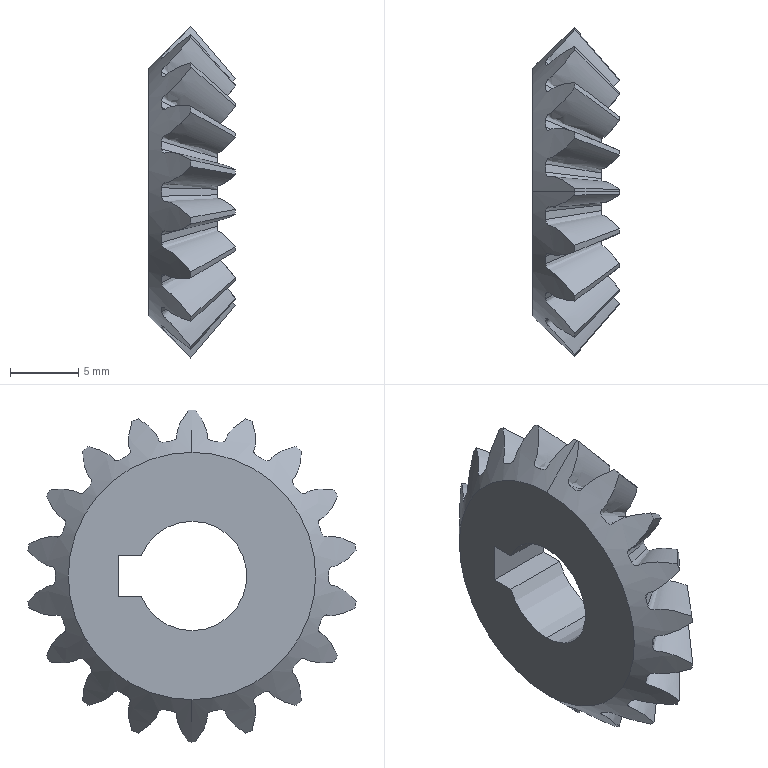Part | SolidWorks | features 3DProfileFeature 12, ICE 2, BlendCut 1, CirPattern 1, RefAxis 1, Revolution 1 | 1 solid | 102 faces | box 6.349 x 23.982 x 24.268 mm | volume 1239 mm3 | cone 40 | spline 36 | plane 23 | cylinder 3 | commonest cylinder face diameters 8 x3